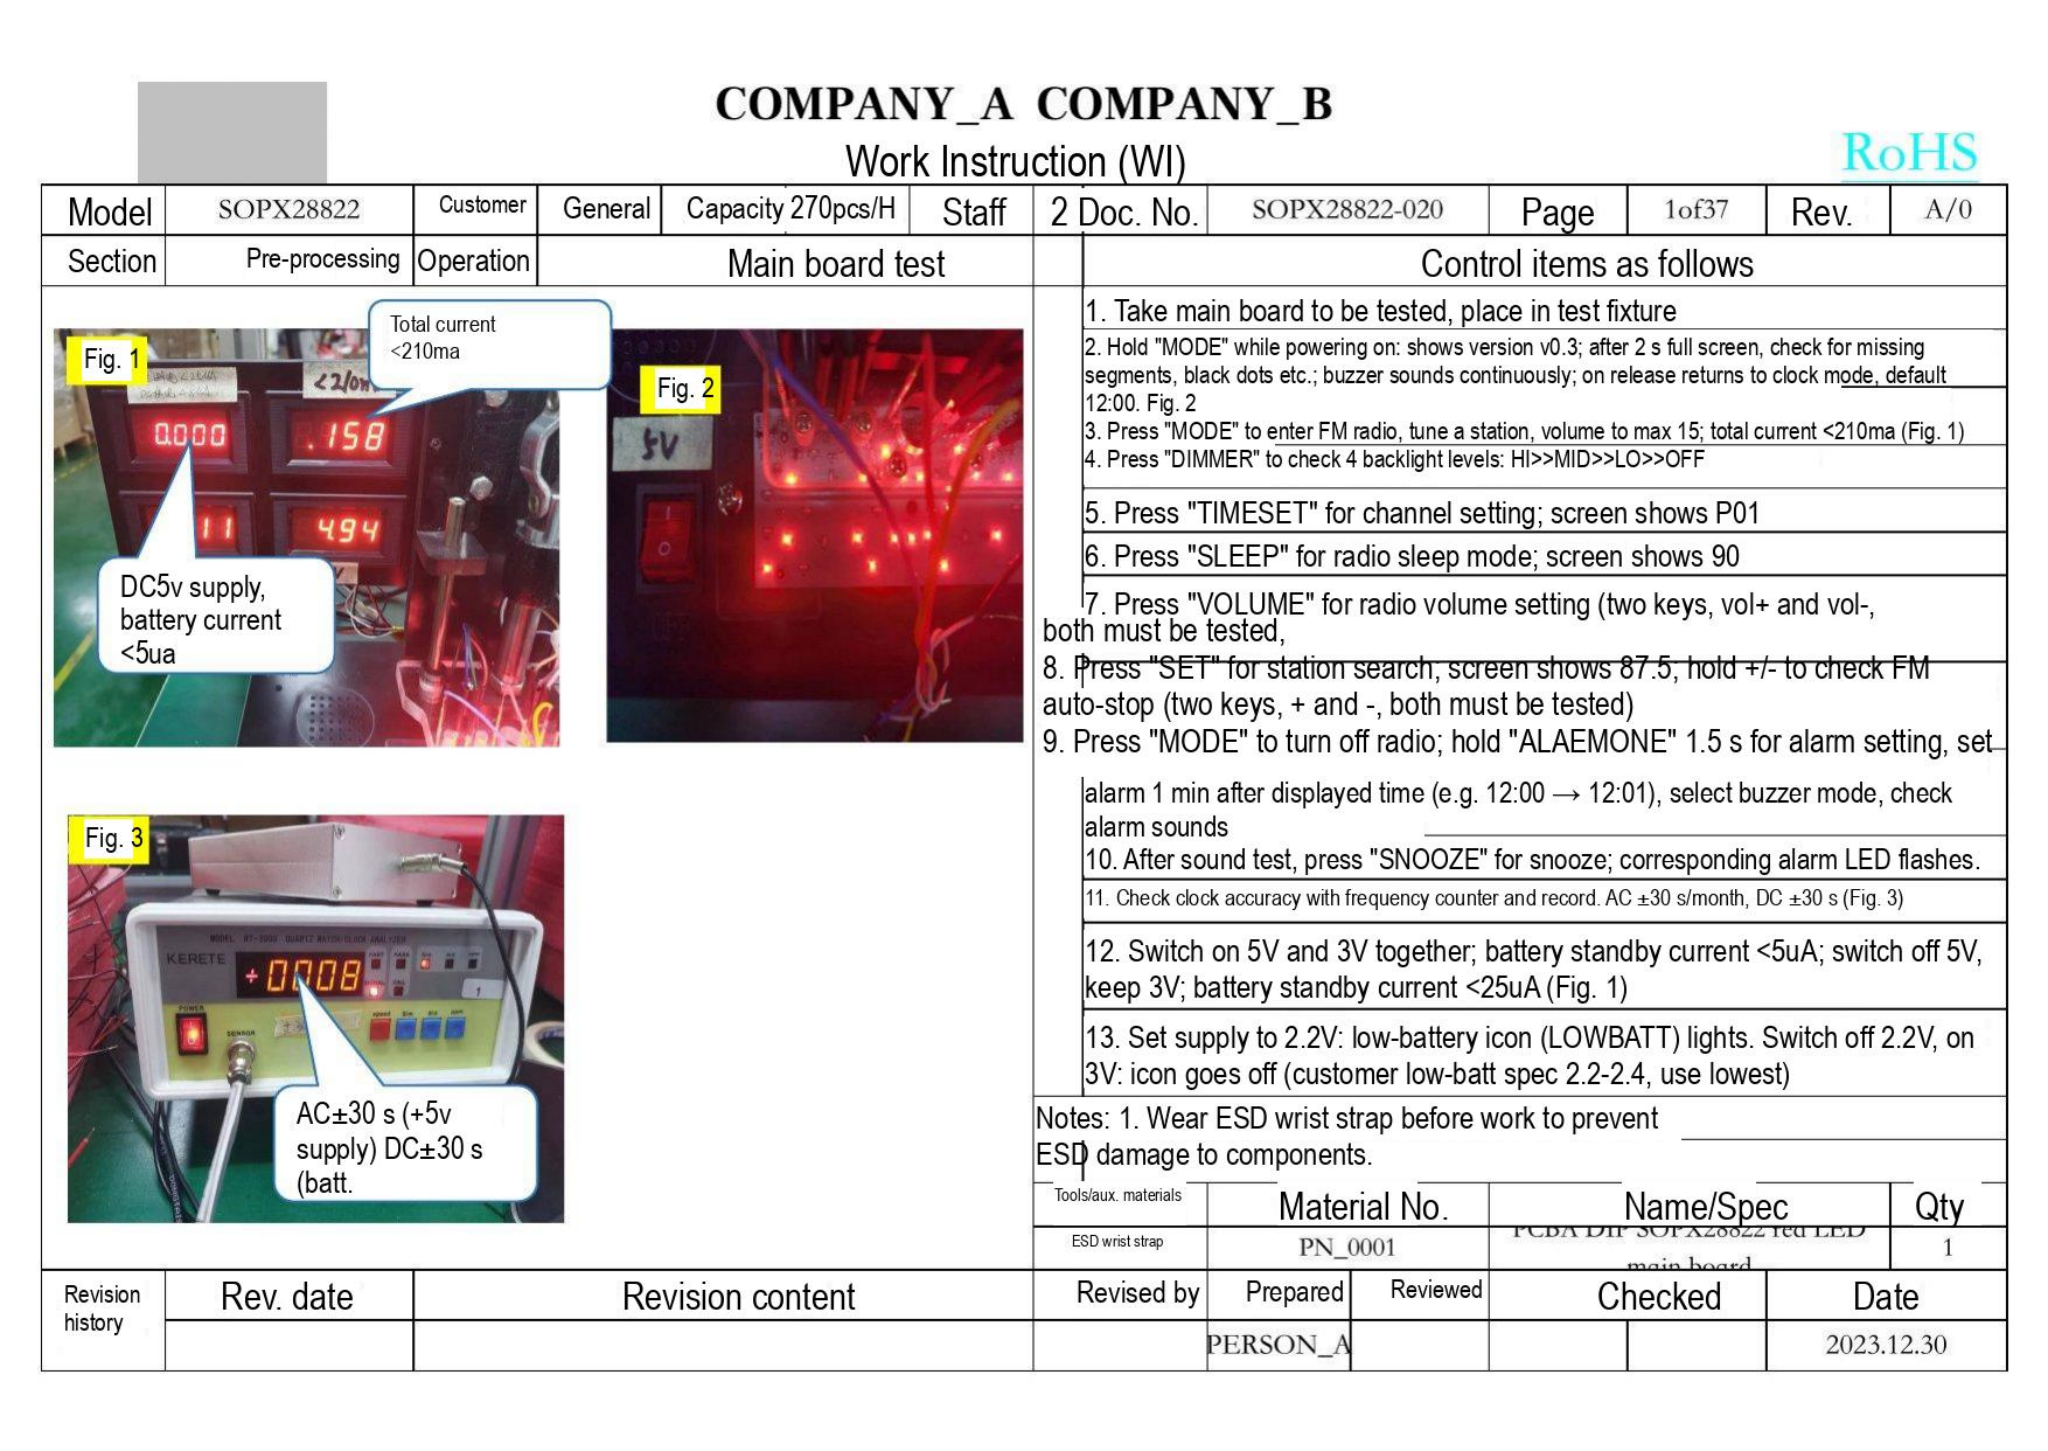COMPANY_A COMPANY_B
Work Instruction (WI)
RoHS

| Model | SOPX28822 | Customer | General | Capacity 270pcs/H | Staff | 2 Doc. No. | SOPX28822-020 | Page | 1of37 | Rev. | A/0 |
|---|---|---|---|---|---|---|---|---|---|---|---|
| Section | Pre-processing | Operation | Main board test | | | | | | | | |

Total current <210ma

Fig. 1

<210

0.000

.158

11

494

DC5v supply, battery current <5ua

Fig. 2

5V

Fig. 3

KERETE

+0008

AC±30 s (+5v supply) DC±30 s (batt.

Control items as follows

1. Take main board to be tested, place in test fixture
2. Hold "MODE" while powering on: shows version v0.3; after 2 s full screen, check for missing segments, black dots etc.; buzzer sounds continuously; on release returns to clock mode, default 12:00. Fig. 2
3. Press "MODE" to enter FM radio, tune a station, volume to max 15; total current <210ma (Fig. 1)
4. Press "DIMMER" to check 4 backlight levels: HI>>MID>>LO>>OFF
5. Press "TIMESET" for channel setting; screen shows P01
6. Press "SLEEP" for radio sleep mode; screen shows 90
7. Press "VOLUME" for radio volume setting (two keys, vol+ and vol-, both must be tested,
8. Press "SET" for station search, screen shows 87.5, hold +/- to check FM auto-stop (two keys, + and -, both must be tested)
9. Press "MODE" to turn off radio; hold "ALAEMONE" 1.5 s for alarm setting, set alarm 1 min after displayed time (e.g. 12:00 → 12:01), select buzzer mode, check alarm sounds
10. After sound test, press "SNOOZE" for snooze; corresponding alarm LED flashes.
11. Check clock accuracy with frequency counter and record. AC ±30 s/month, DC ±30 s (Fig. 3)
12. Switch on 5V and 3V together; battery standby current <5uA; switch off 5V, keep 3V; battery standby current <25uA (Fig. 1)
13. Set supply to 2.2V: low-battery icon (LOWBATT) lights. Switch off 2.2V, on 3V: icon goes off (customer low-batt spec 2.2-2.4, use lowest)

Notes: 1. Wear ESD wrist strap before work to prevent ESD damage to components.

| Tools/aux. materials | Material No. | Name/Spec | Qty |
|---|---|---|---|
| ESD wrist strap | PN_0001 | PCBA DIP SOPX28822 red LED main board | 1 |

| Revision history | Rev. date | Revision content | Revised by | Prepared | Reviewed | Checked | Date |
|---|---|---|---|---|---|---|---|
| | | | | PERSON_A | | | 2023.12.30 |
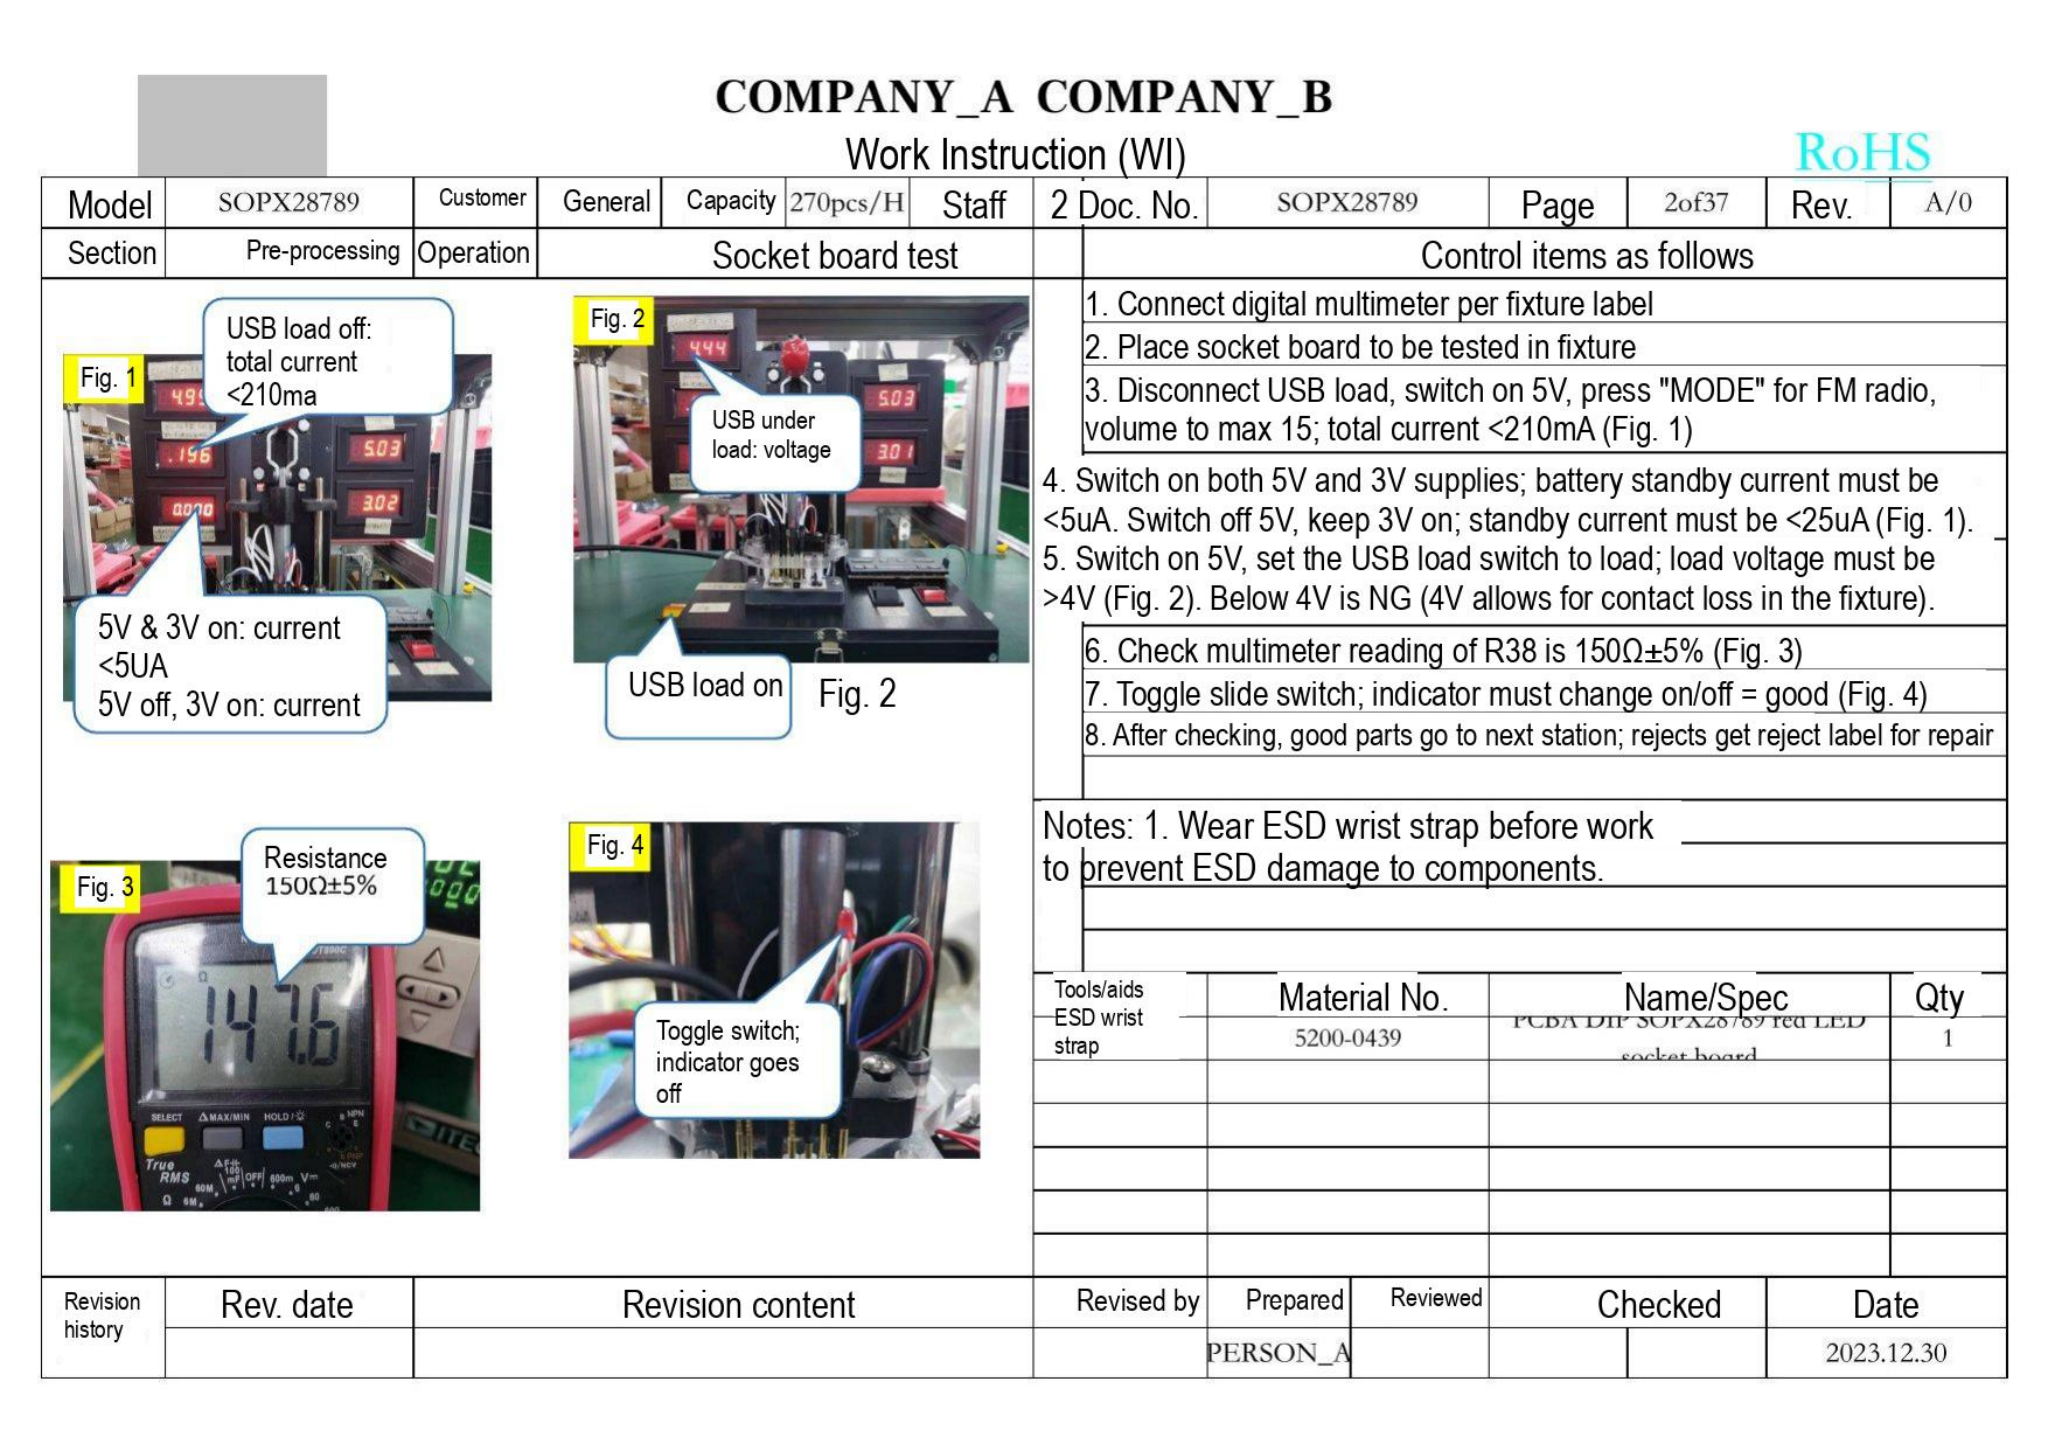COMPANY_A COMPANY_B

Work Instruction (WI)

RoHS

| Model | SOPX28789 | Customer | General | Capacity | 270pcs/H | Staff | 2 | Doc. No. | SOPX28789 | Page | 2of37 | Rev. | A/0 |
|---|---|---|---|---|---|---|---|---|---|---|---|---|---|
| Section | Pre-processing | Operation | Socket board test | | | | | Control items as follows | | | | | |

Fig. 1

USB load off: total current <210ma

5V & 3V on: current <5UA
5V off, 3V on: current

Fig. 2

USB under load: voltage

USB load on

Fig. 2

Fig. 3

Resistance 150Ω±5%

Fig. 4

Toggle switch; indicator goes off

Control items as follows

1. Connect digital multimeter per fixture label
2. Place socket board to be tested in fixture
3. Disconnect USB load, switch on 5V, press "MODE" for FM radio, volume to max 15; total current <210mA (Fig. 1)
4. Switch on both 5V and 3V supplies; battery standby current must be <5uA. Switch off 5V, keep 3V on; standby current must be <25uA (Fig. 1).
5. Switch on 5V, set the USB load switch to load; load voltage must be >4V (Fig. 2). Below 4V is NG (4V allows for contact loss in the fixture).
6. Check multimeter reading of R38 is 150Ω±5% (Fig. 3)
7. Toggle slide switch; indicator must change on/off = good (Fig. 4)
8. After checking, good parts go to next station; rejects get reject label for repair

Notes: 1. Wear ESD wrist strap before work to prevent ESD damage to components.

| Tools/aids | Material No. | Name/Spec | Qty |
|---|---|---|---|
| ESD wrist strap | 5200-0439 | PCBA DIP SOPX28789 red LED socket board | 1 |
| | | | |
| | | | |
| | | | |
| | | | |
| | | | |

| Revision history | Rev. date | Revision content | Revised by | Prepared | Reviewed | Checked | Date |
|---|---|---|---|---|---|---|---|
| | | | | PERSON_A | | | 2023.12.30 |
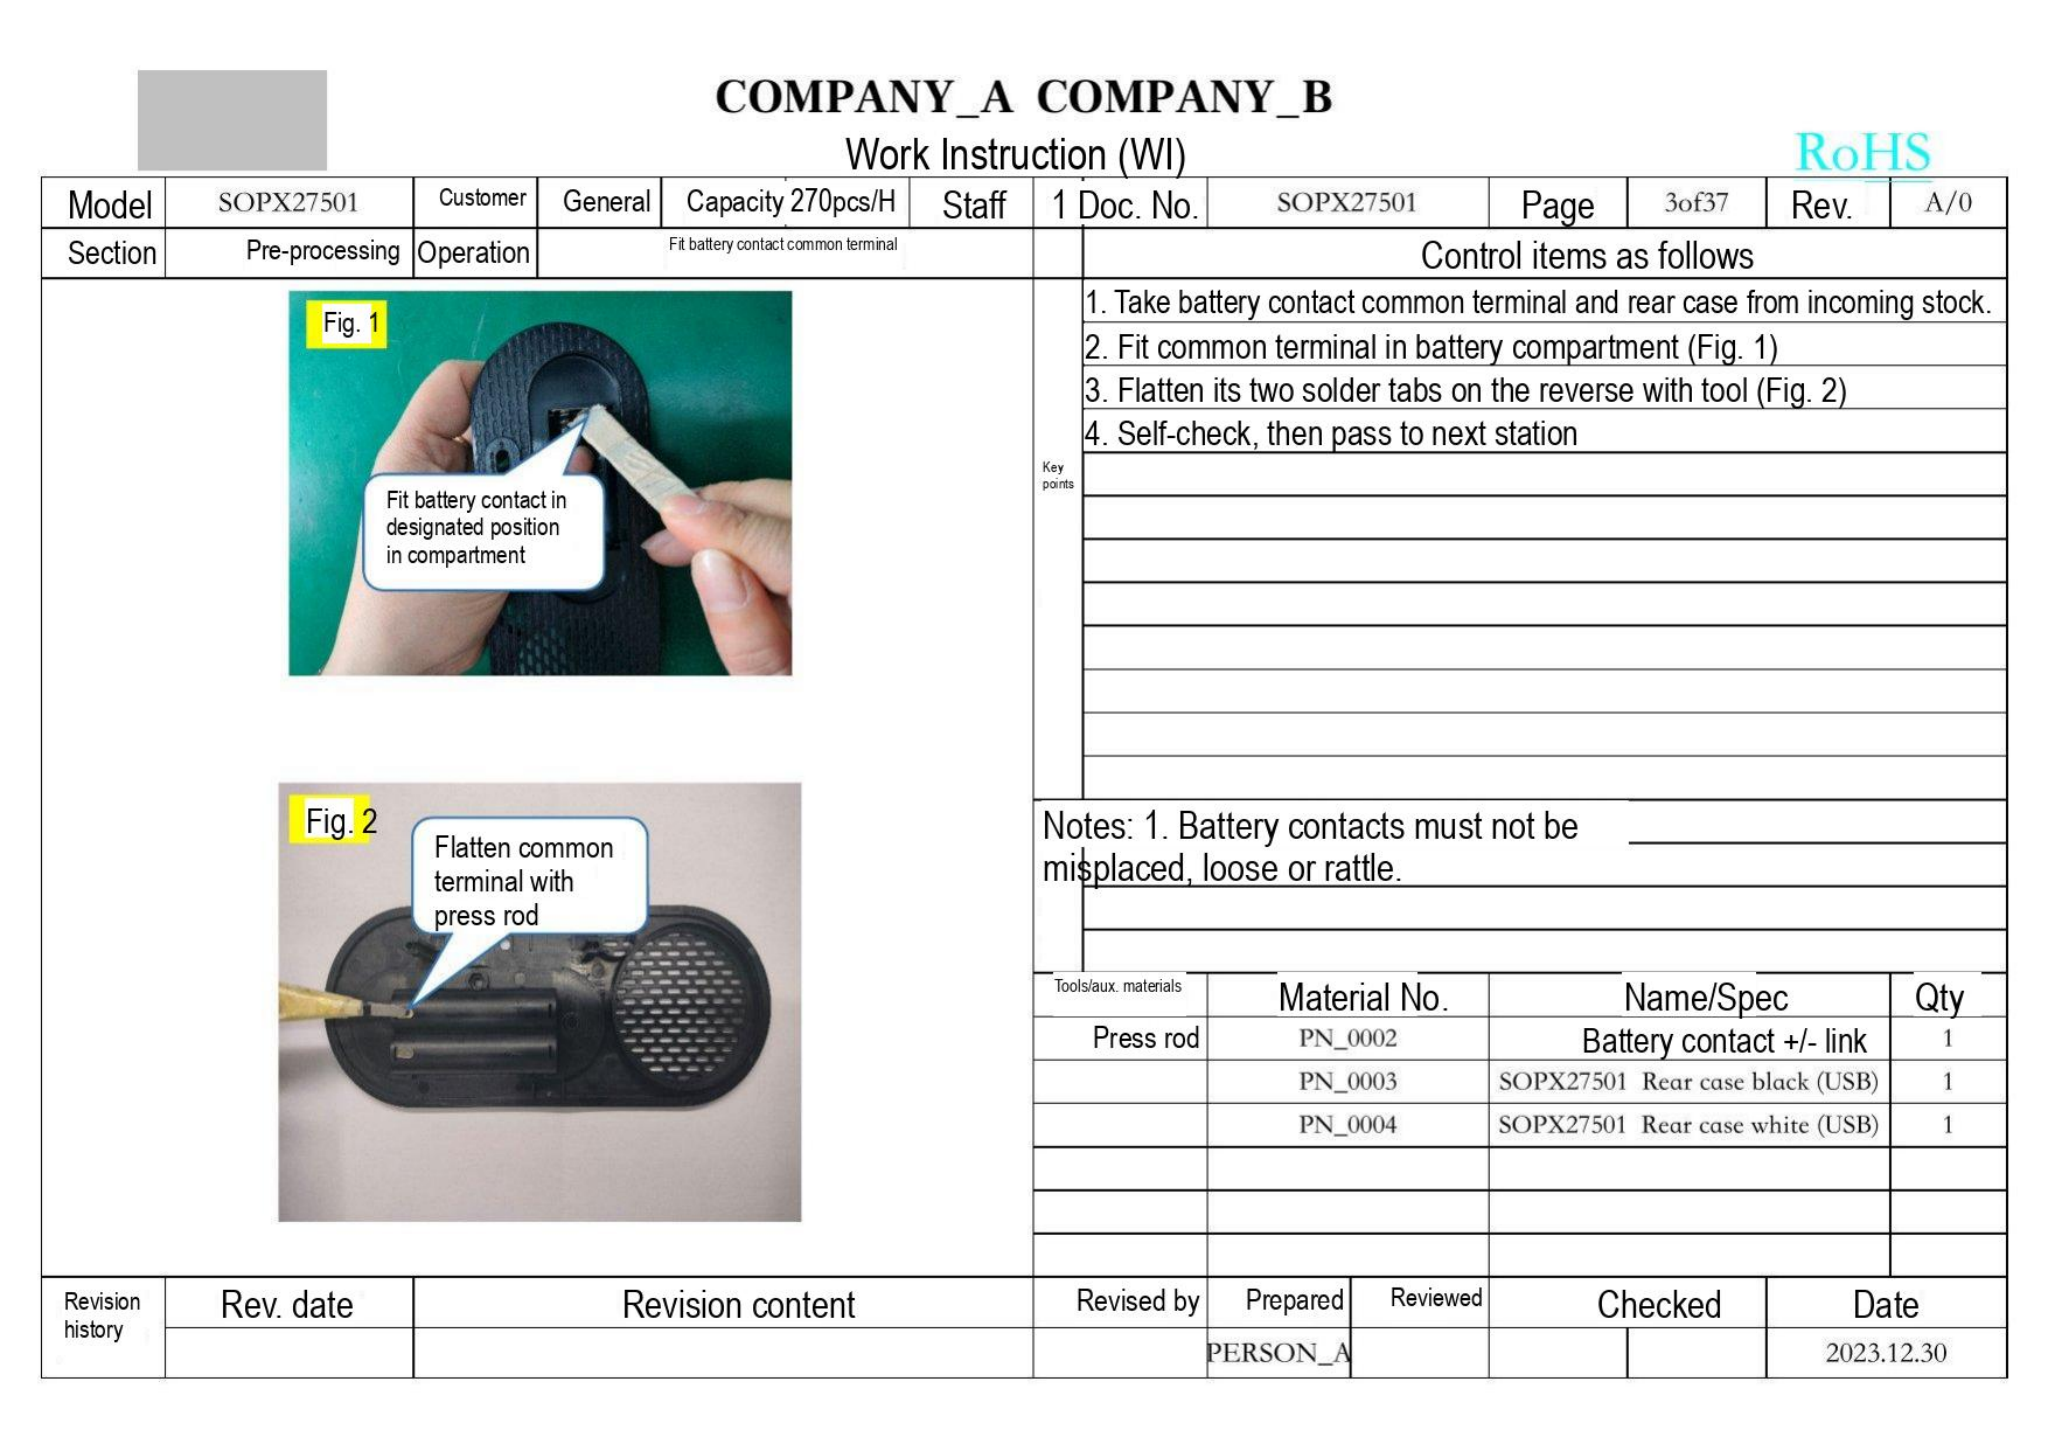COMPANY_A COMPANY_B
Work Instruction (WI)
RoHS

| Model | SOPX27501 | Customer | General | Capacity 270pcs/H | Staff | 1 | Doc. No. | SOPX27501 | Page | 3of37 | Rev. | A/0 |
|---|---|---|---|---|---|---|---|---|---|---|---|---|
| Section | Pre-processing | Operation | Fit battery contact common terminal | | | | | | | | | |

Fig. 1
Fit battery contact in designated position in compartment

Fig. 2
Flatten common terminal with press rod

Control items as follows

Key points
1. Take battery contact common terminal and rear case from incoming stock.
2. Fit common terminal in battery compartment (Fig. 1)
3. Flatten its two solder tabs on the reverse with tool (Fig. 2)
4. Self-check, then pass to next station

Notes: 1. Battery contacts must not be misplaced, loose or rattle.

| Tools/aux. materials | Material No. | Name/Spec | Qty |
|---|---|---|---|
| Press rod | PN_0002 | Battery contact +/- link | 1 |
| | PN_0003 | SOPX27501 Rear case black (USB) | 1 |
| | PN_0004 | SOPX27501 Rear case white (USB) | 1 |
| | | | |
| | | | |
| | | | |

| Revision history | Rev. date | Revision content | Revised by | Prepared | Reviewed | Checked | Date |
|---|---|---|---|---|---|---|---|
| | | | | PERSON_A | | | 2023.12.30 |
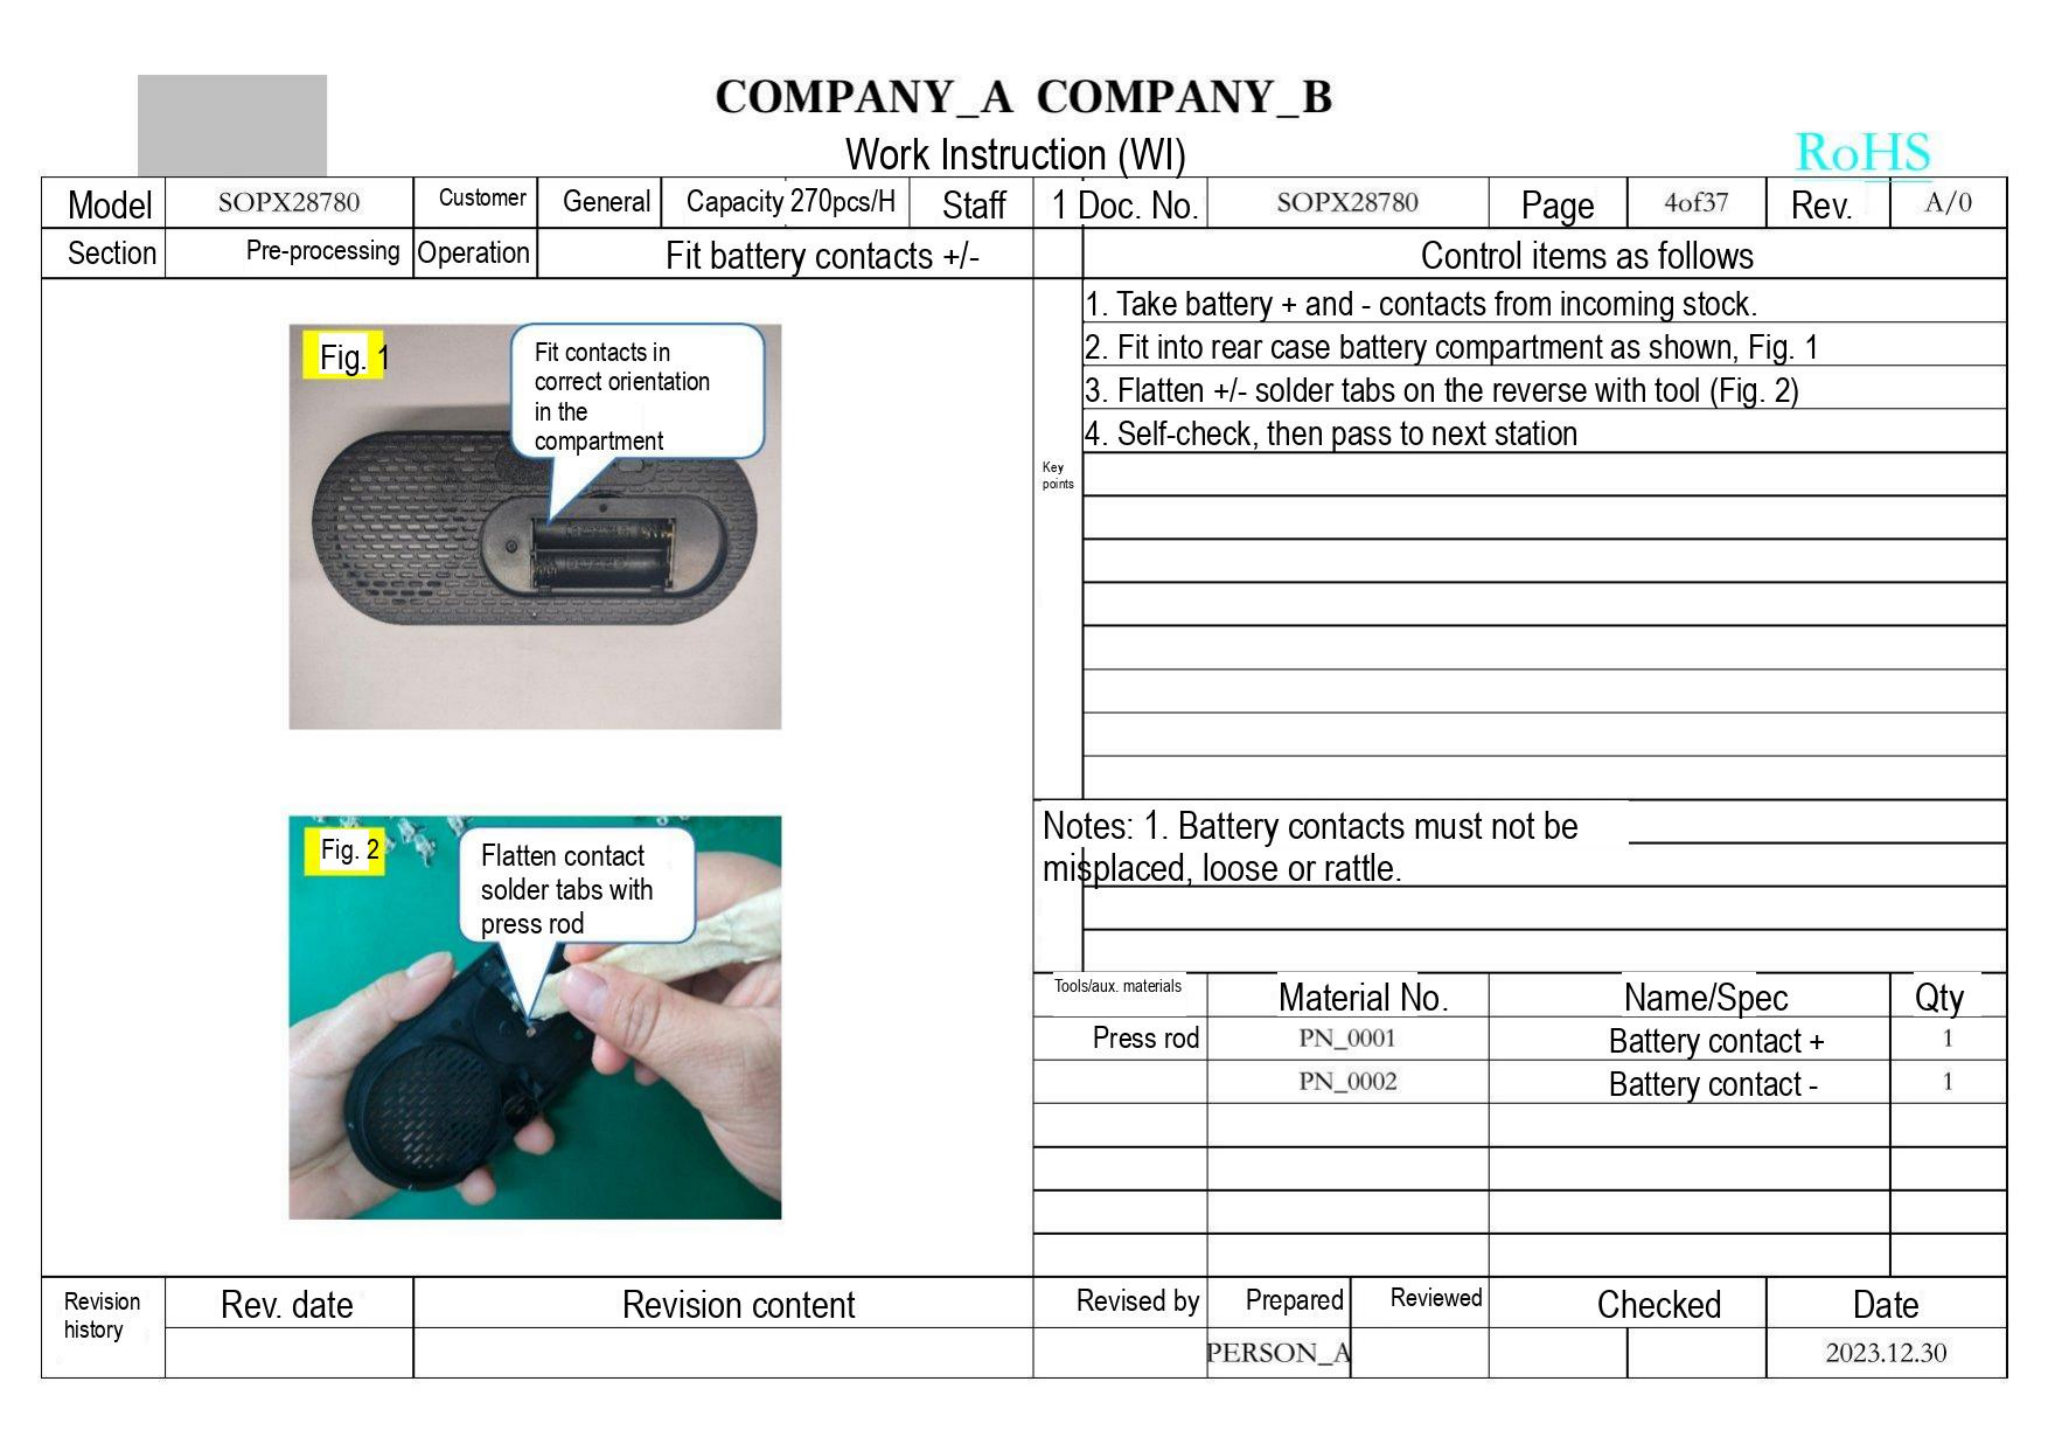COMPANY_A COMPANY_B
Work Instruction (WI)
RoHS

| Model | SOPX28780 | Customer | General | Capacity 270pcs/H | Staff | 1 | Doc. No. | SOPX28780 | Page | 4of37 | Rev. | A/0 |
|---|---|---|---|---|---|---|---|---|---|---|---|---|
| Section | Pre-processing | Operation | Fit battery contacts +/- | | | | | | | | | |

Fig. 1
Fit contacts in correct orientation in the compartment

Fig. 2
Flatten contact solder tabs with press rod

Control items as follows

Key points
1. Take battery + and - contacts from incoming stock.
2. Fit into rear case battery compartment as shown, Fig. 1
3. Flatten +/- solder tabs on the reverse with tool (Fig. 2)
4. Self-check, then pass to next station

Notes: 1. Battery contacts must not be misplaced, loose or rattle.

| Tools/aux. materials | Material No. | Name/Spec | Qty |
|---|---|---|---|
| Press rod | PN_0001 | Battery contact + | 1 |
| | PN_0002 | Battery contact - | 1 |
| | | | |
| | | | |
| | | | |
| | | | |

| Revision history | Rev. date | Revision content | Revised by | Prepared | Reviewed | Checked | Date |
|---|---|---|---|---|---|---|---|
| | | | | PERSON_A | | | 2023.12.30 |
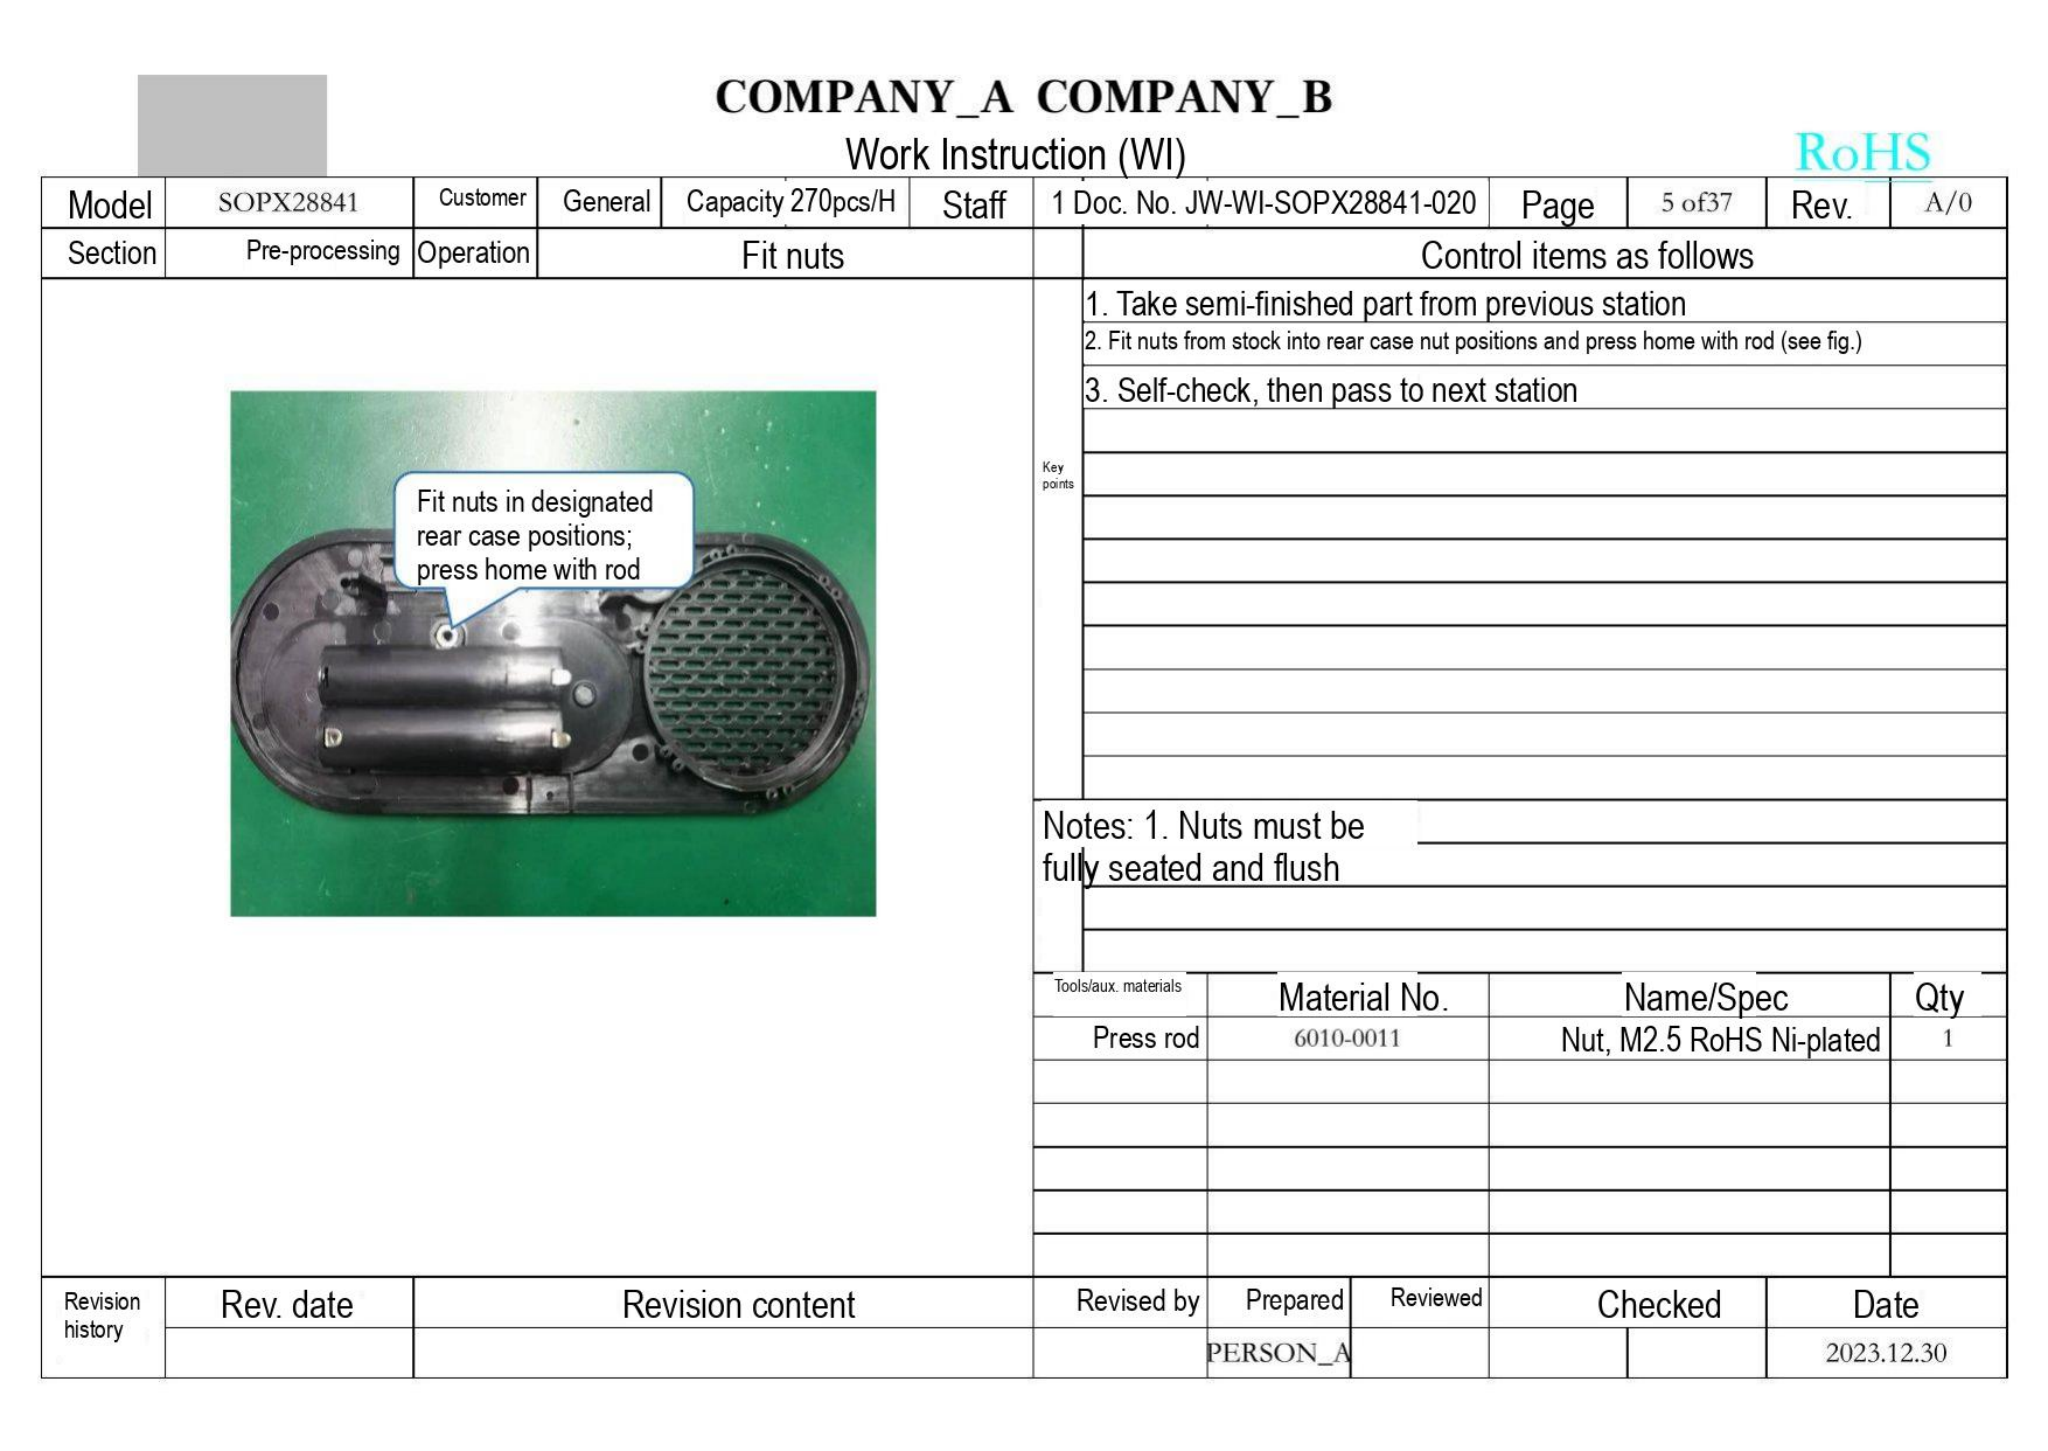COMPANY_A COMPANY_B
Work Instruction (WI)
RoHS

| Model | SOPX28841 | Customer | General | Capacity 270pcs/H | Staff | 1 Doc. No. JW-WI-SOPX28841-020 | Page | 5 of37 | Rev. | A/0 |
|---|---|---|---|---|---|---|---|---|---|---|
| Section | Pre-processing | Operation | Fit nuts | | | | | | | |

Fit nuts in designated rear case positions; press home with rod

Control items as follows

| Key points | |
|---|---|
| | 1. Take semi-finished part from previous station |
| | 2. Fit nuts from stock into rear case nut positions and press home with rod (see fig.) |
| | 3. Self-check, then pass to next station |

Notes: 1. Nuts must be fully seated and flush

| Tools/aux. materials | Material No. | Name/Spec | Qty |
|---|---|---|---|
| Press rod | 6010-0011 | Nut, M2.5 RoHS Ni-plated | 1 |

| Revision history | Rev. date | Revision content | Revised by | Prepared | Reviewed | Checked | Date |
|---|---|---|---|---|---|---|---|
| | | | | PERSON_A | | | 2023.12.30 |
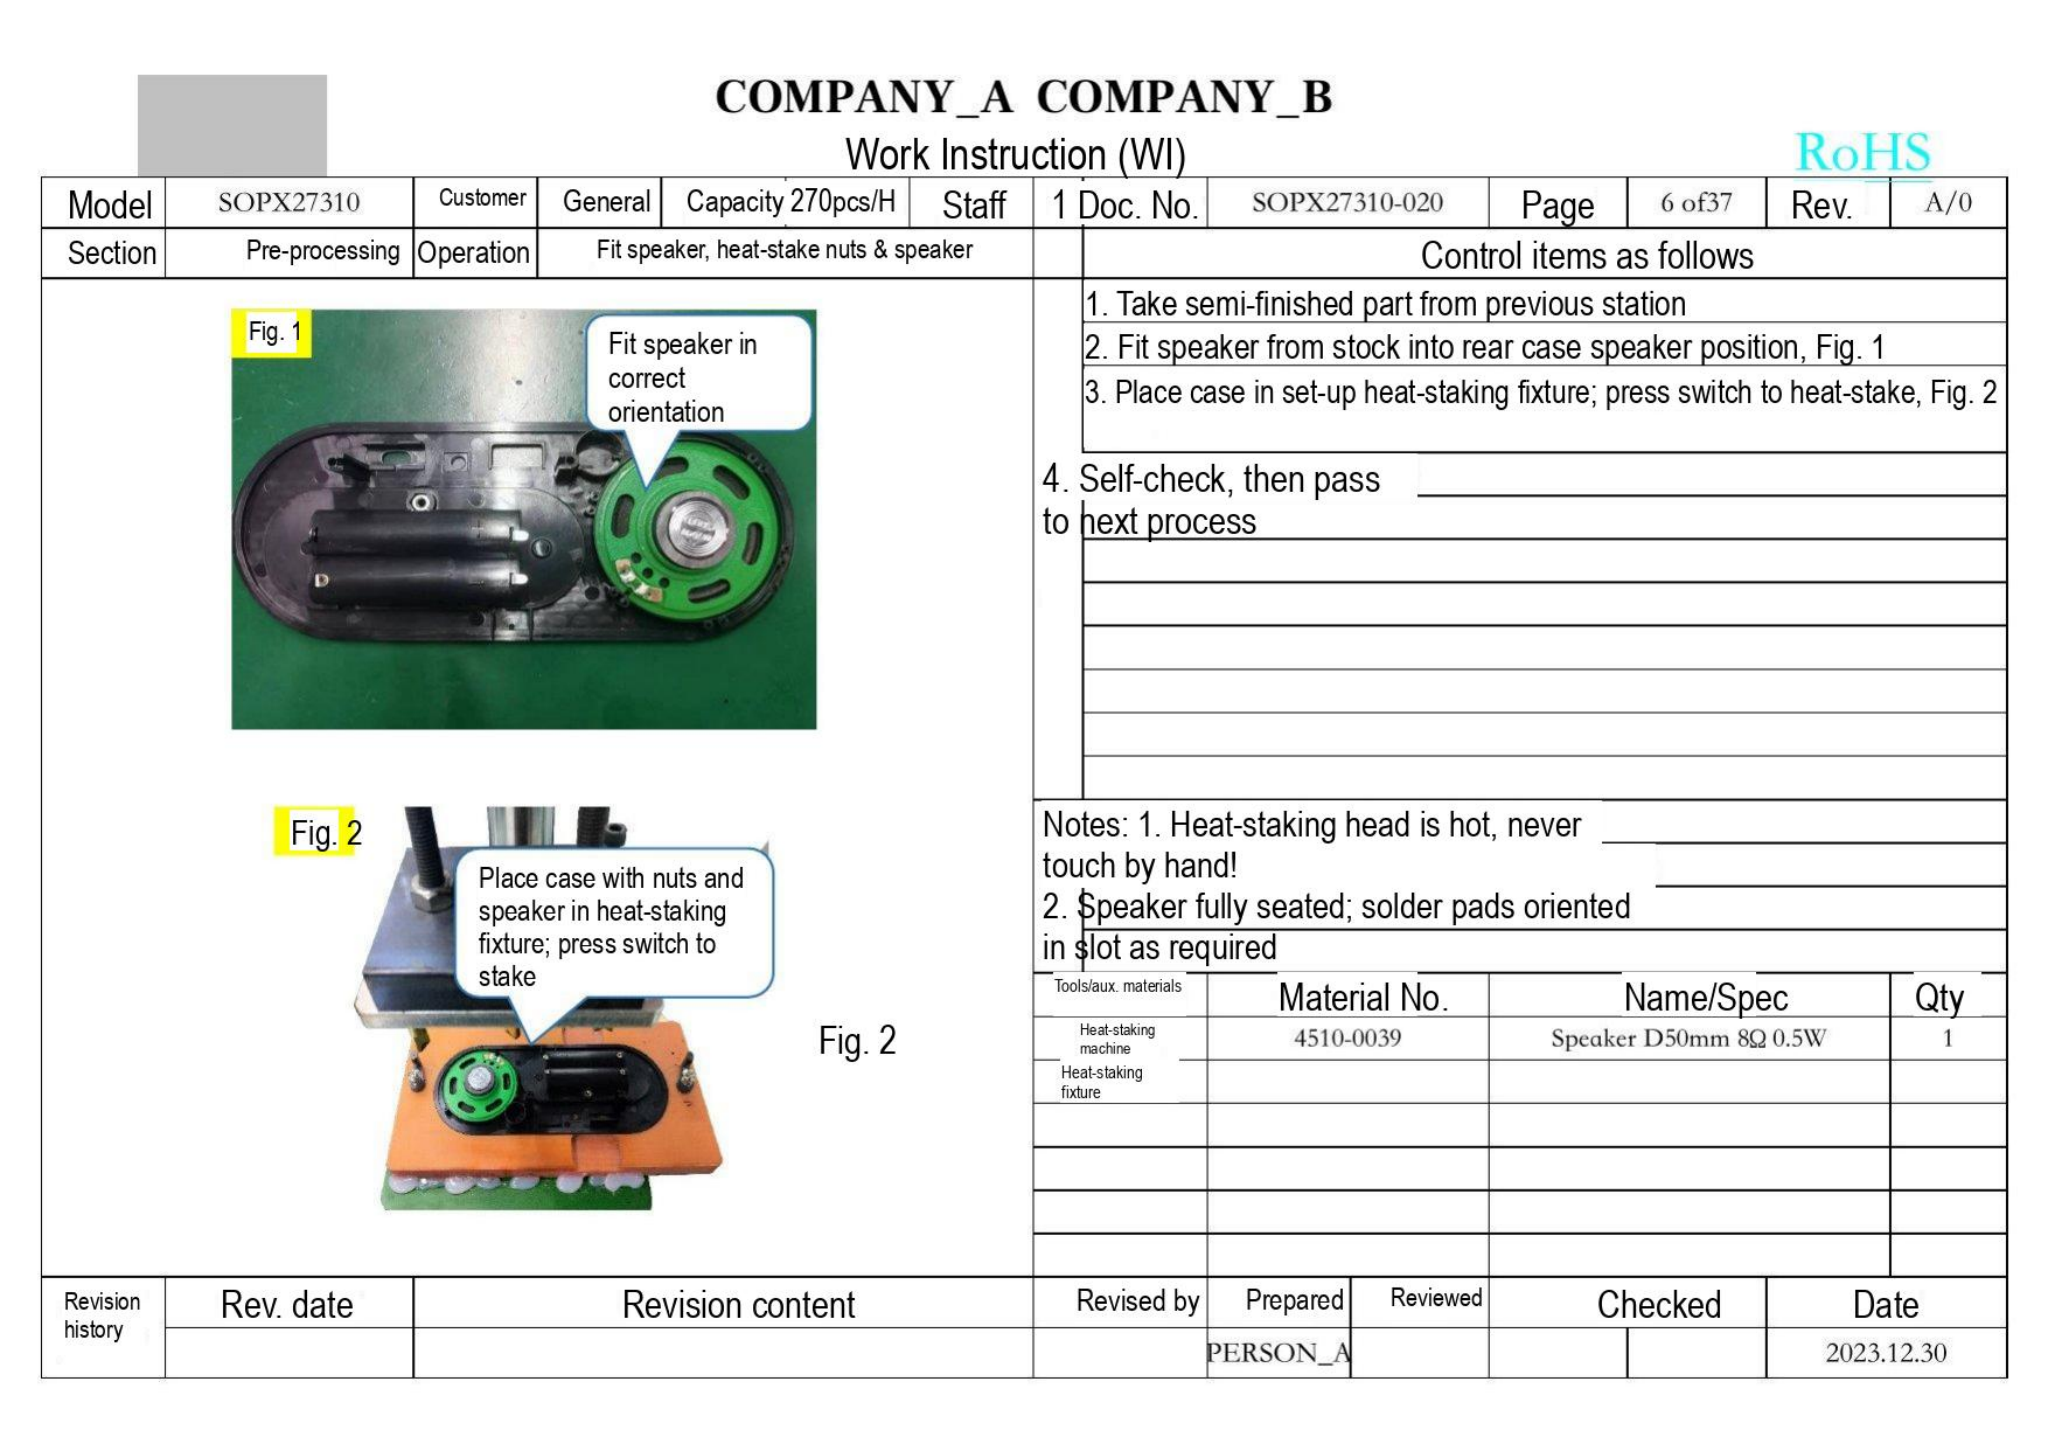COMPANY_A COMPANY_B
Work Instruction (WI)
RoHS

| Model | SOPX27310 | Customer | General | Capacity 270pcs/H | Staff | 1 | Doc. No. | SOPX27310-020 | Page | 6 of37 | Rev. | A/0 |
|---|---|---|---|---|---|---|---|---|---|---|---|---|
| Section | Pre-processing | Operation | Fit speaker, heat-stake nuts & speaker | | | | | | | | | |

Fig. 1
Fit speaker in correct orientation

Fig. 2
Place case with nuts and speaker in heat-staking fixture; press switch to stake

Fig. 2

Control items as follows
1. Take semi-finished part from previous station
2. Fit speaker from stock into rear case speaker position, Fig. 1
3. Place case in set-up heat-staking fixture; press switch to heat-stake, Fig. 2
4. Self-check, then pass to next process

Notes: 1. Heat-staking head is hot, never touch by hand!
2. Speaker fully seated; solder pads oriented in slot as required

| Tools/aux. materials | Material No. | Name/Spec | Qty |
|---|---|---|---|
| Heat-staking machine | 4510-0039 | Speaker D50mm 8Ω 0.5W | 1 |
| Heat-staking fixture | | | |

| Revision history | Rev. date | Revision content | Revised by | Prepared | Reviewed | Checked | Date |
|---|---|---|---|---|---|---|---|
| | | | | PERSON_A | | | 2023.12.30 |
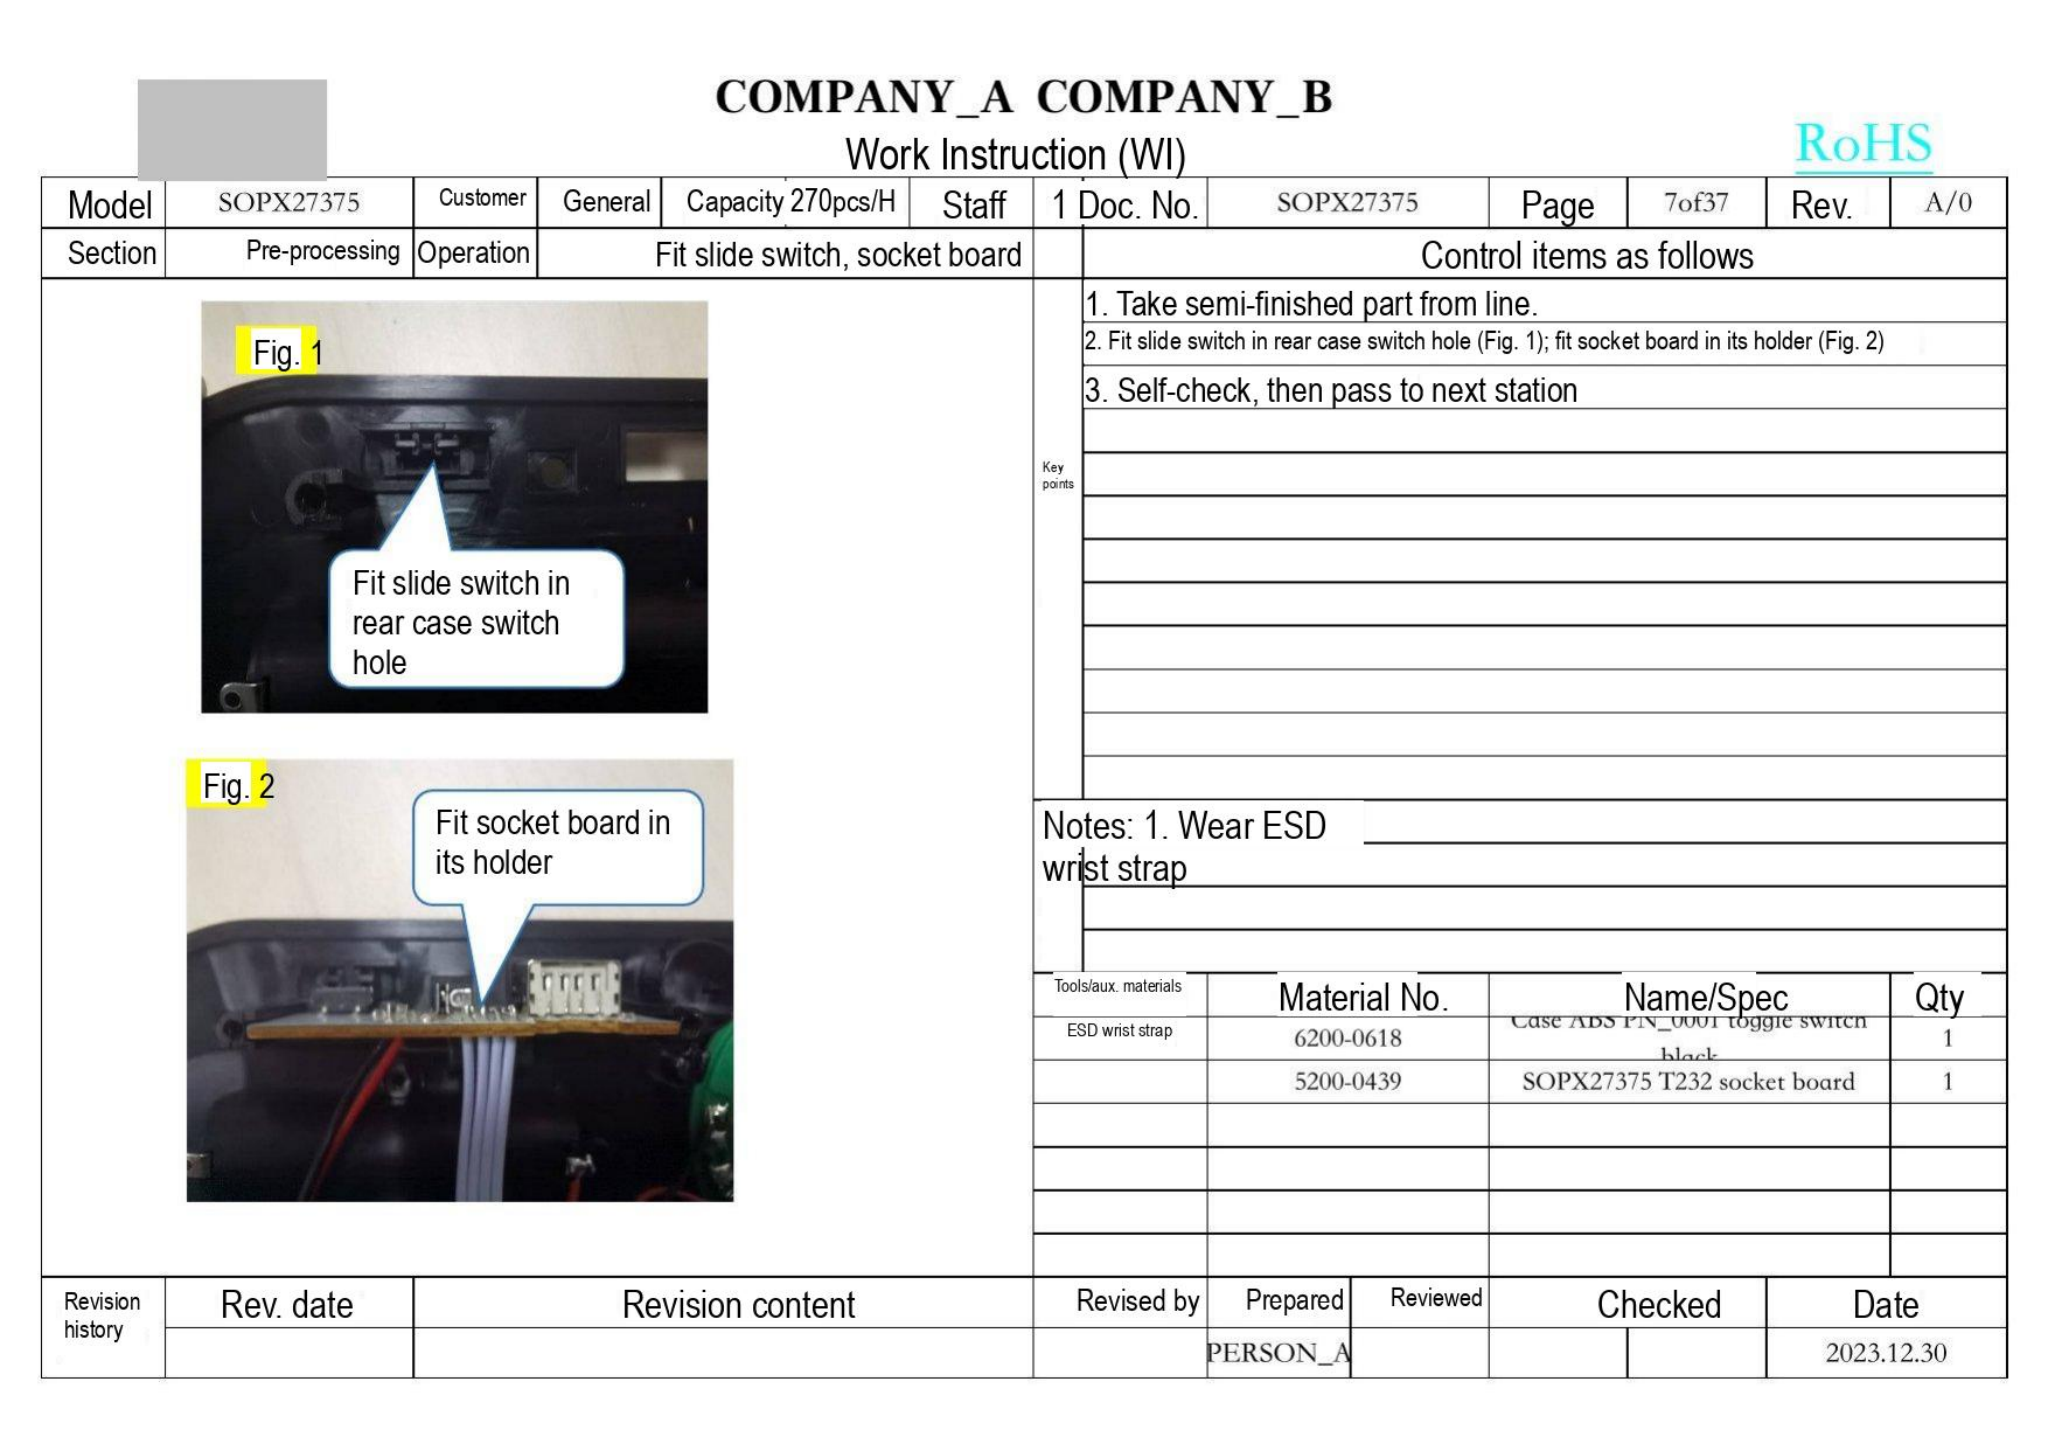COMPANY_A COMPANY_B

Work Instruction (WI)

RoHS

| Model | SOPX27375 | Customer | General | Capacity 270pcs/H | Staff | 1 | Doc. No. | SOPX27375 | Page | 7of37 | Rev. | A/0 |
|---|---|---|---|---|---|---|---|---|---|---|---|---|
| Section | Pre-processing | Operation | Fit slide switch, socket board | | | | | | | | | |

Fig. 1

Fit slide switch in rear case switch hole

Fig. 2

Fit socket board in its holder

| | Control items as follows |
|---|---|
| Key points | 1. Take semi-finished part from line. |
| | 2. Fit slide switch in rear case switch hole (Fig. 1); fit socket board in its holder (Fig. 2) |
| | 3. Self-check, then pass to next station |

Notes: 1. Wear ESD wrist strap

| Tools/aux. materials | Material No. | Name/Spec | Qty |
|---|---|---|---|
| ESD wrist strap | 6200-0618 | Case ABS PN_0001 toggle switch black | 1 |
| | 5200-0439 | SOPX27375 T232 socket board | 1 |

| Revision history | Rev. date | Revision content | Revised by | Prepared | Reviewed | Checked | Date |
|---|---|---|---|---|---|---|---|
| | | | | PERSON_A | | | 2023.12.30 |